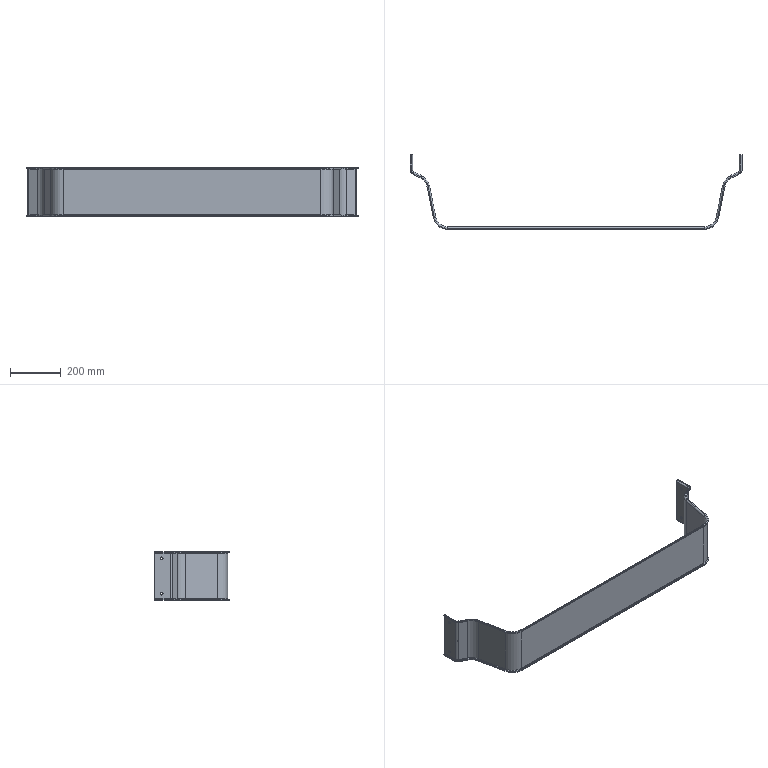Part | SolidWorks | features ICE 13, Fillet 9, HoleWzd 2, Extrusion 1 | 1 solid | 118 faces | box 1308 x 294 x 192 mm | volume 1374323 mm3 | cylinder 60 | plane 34 | torus 24 | commonest cylinder face diameters 12 x16 4 x14 10 x8 32 x4 88 x4 100 x4